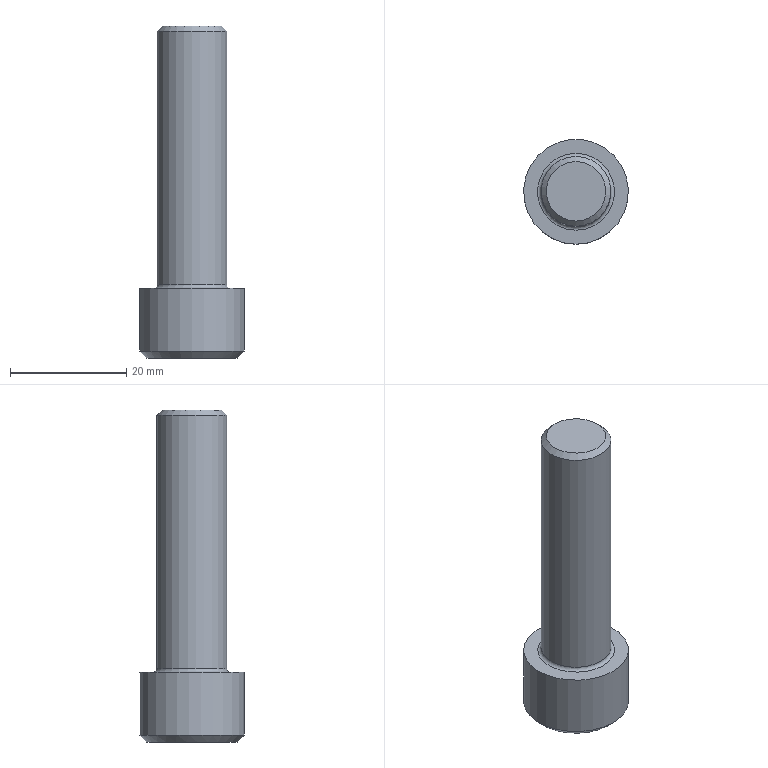Part | STEP file | solid 68 | 1 solid | 21 faces | box 18 x 18 x 57 mm | volume 7571 mm3 | plane 10 | sphere 6 | cylinder 2 | cone 2 | torus 1 | commonest cylinder face diameters 12 x1 18 x1